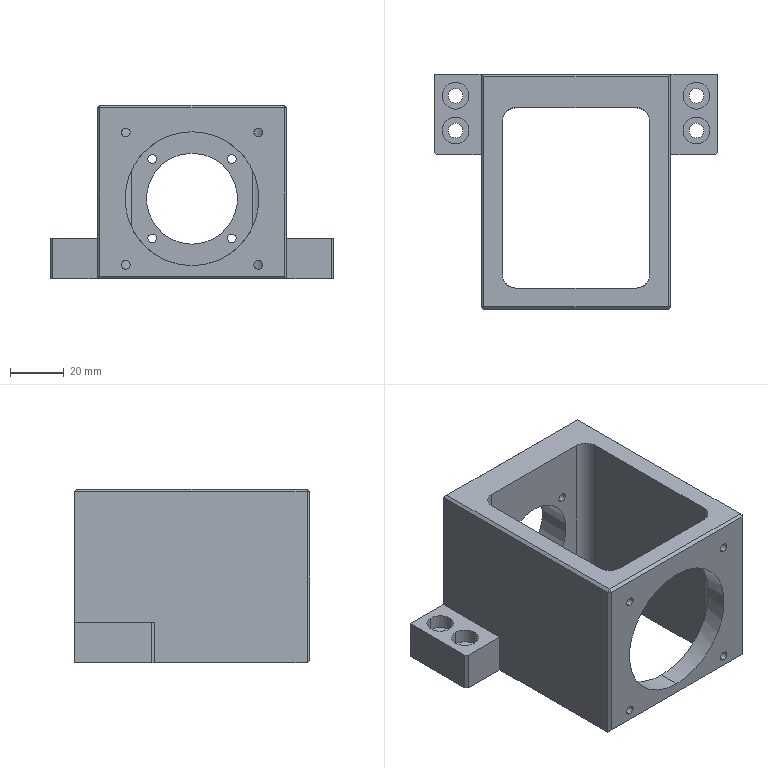Part | 1 solid | 72 faces | box 106 x 88 x 65 mm | volume 151217 mm3 | cylinder 40 | plane 32 | commonest cylinder face diameters 3.3 x16 10 x12 5.5 x8 34 x2 50.1 x2